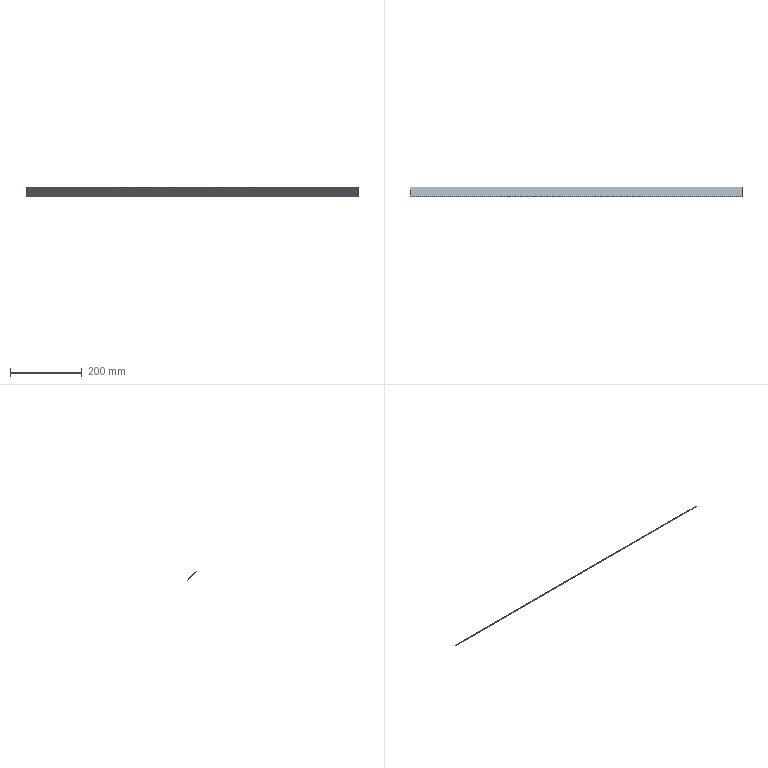Part | SolidWorks | features BaseBody 1 | 1 solid | 6 faces | box 924.6 x 26.8 x 26.8 mm | volume 50484 mm3 | plane 6
STEP:
#1=CARTESIAN_POINT('',(924.6,26.8,2.121));
#2=VERTEX_POINT('',#1);
#3=CARTESIAN_POINT('',(924.6,26.8,0.));
#4=VERTEX_POINT('',#3);
#5=CARTESIAN_POINT('',(924.6,26.8,0.));
#6=DIRECTION('',(0.,0.,-1.));
#7=VECTOR('',#6,1000.);
#8=LINE('',#5,#7);
#9=EDGE_CURVE('',#2,#4,#8,.T.);
#10=ORIENTED_EDGE('',*,*,#9,.T.);
#11=CARTESIAN_POINT('',(0.,26.8,0.));
#12=VERTEX_POINT('',#11);
#13=CARTESIAN_POINT('',(924.6,26.8,0.));
#14=DIRECTION('',(-1.,0.,0.));
#15=VECTOR('',#14,1000.);
#16=LINE('',#13,#15);
#17=EDGE_CURVE('',#4,#12,#16,.T.);
#18=ORIENTED_EDGE('',*,*,#17,.T.);
#19=CARTESIAN_POINT('',(0.,26.8,2.121));
#20=VERTEX_POINT('',#19);
#21=CARTESIAN_POINT('',(0.,26.8,0.));
#22=DIRECTION('',(0.,0.,1.));
#23=VECTOR('',#22,1000.);
#24=LINE('',#21,#23);
#25=EDGE_CURVE('',#12,#20,#24,.T.);
#26=ORIENTED_EDGE('',*,*,#25,.T.);
#27=CARTESIAN_POINT('',(924.6,26.8,2.121));
#28=DIRECTION('',(-1.,0.,0.));
#29=VECTOR('',#28,1000.);
#30=LINE('',#27,#29);
#31=EDGE_CURVE('',#2,#20,#30,.T.);
#32=ORIENTED_EDGE('',*,*,#31,.F.);
#33=EDGE_LOOP('',(#10,#18,#26,#32));
#34=FACE_OUTER_BOUND('',#33,.T.);
#35=CARTESIAN_POINT('',(0.,26.8,0.));
#36=DIRECTION('',(0.,-1.,0.));
#37=DIRECTION('',(0.,0.,-1.));
#38=AXIS2_PLACEMENT_3D('',#35,#36,#37);
#39=PLANE('',#38);
#40=ADVANCED_FACE('',(#34),#39,.F.);
#41=CARTESIAN_POINT('',(0.,0.,26.8));
#42=VERTEX_POINT('',#41);
#43=CARTESIAN_POINT('',(0.,2.121,26.8));
#44=VERTEX_POINT('',#43);
#45=CARTESIAN_POINT('',(0.,0.,26.8));
#46=DIRECTION('',(0.,1.,0.));
#47=VECTOR('',#46,1000.);
#48=LINE('',#45,#47);
#49=EDGE_CURVE('',#42,#44,#48,.T.);
#50=ORIENTED_EDGE('',*,*,#49,.F.);
#51=CARTESIAN_POINT('',(924.6,0.,26.8));
#52=VERTEX_POINT('',#51);
#53=CARTESIAN_POINT('',(924.6,0.,26.8));
#54=DIRECTION('',(-1.,0.,0.));
#55=VECTOR('',#54,1000.);
#56=LINE('',#53,#55);
#57=EDGE_CURVE('',#52,#42,#56,.T.);
#58=ORIENTED_EDGE('',*,*,#57,.F.);
#59=CARTESIAN_POINT('',(924.6,2.121,26.8));
#60=VERTEX_POINT('',#59);
#61=CARTESIAN_POINT('',(924.6,0.,26.8));
#62=DIRECTION('',(0.,1.,0.));
#63=VECTOR('',#62,1000.);
#64=LINE('',#61,#63);
#65=EDGE_CURVE('',#52,#60,#64,.T.);
#66=ORIENTED_EDGE('',*,*,#65,.T.);
#67=CARTESIAN_POINT('',(924.6,2.121,26.8));
#68=DIRECTION('',(1.,0.,0.));
#69=VECTOR('',#68,1000.);
#70=LINE('',#67,#69);
#71=EDGE_CURVE('',#44,#60,#70,.T.);
#72=ORIENTED_EDGE('',*,*,#71,.F.);
#73=EDGE_LOOP('',(#50,#58,#66,#72));
#74=FACE_OUTER_BOUND('',#73,.T.);
#75=CARTESIAN_POINT('',(0.,0.,26.8));
#76=DIRECTION('',(0.,0.,-1.));
#77=DIRECTION('',(0.,-1.,0.));
#78=AXIS2_PLACEMENT_3D('',#75,#76,#77);
#79=PLANE('',#78);
#80=ADVANCED_FACE('',(#74),#79,.F.);
#81=ORIENTED_EDGE('',*,*,#25,.F.);
#82=CARTESIAN_POINT('',(0.,26.8,0.));
#83=DIRECTION('',(0.,-0.7071,0.7071));
#84=VECTOR('',#83,1000.);
#85=LINE('',#82,#84);
#86=EDGE_CURVE('',#12,#42,#85,.T.);
#87=ORIENTED_EDGE('',*,*,#86,.T.);
#88=ORIENTED_EDGE('',*,*,#49,.T.);
#89=CARTESIAN_POINT('',(0.,27.861,1.061));
#90=DIRECTION('',(0.,-0.7071,0.7071));
#91=VECTOR('',#90,1000.);
#92=LINE('',#89,#91);
#93=EDGE_CURVE('',#20,#44,#92,.T.);
#94=ORIENTED_EDGE('',*,*,#93,.F.);
#95=EDGE_LOOP('',(#81,#87,#88,#94));
#96=FACE_OUTER_BOUND('',#95,.T.);
#97=CARTESIAN_POINT('',(0.,0.,0.));
#98=DIRECTION('',(-1.,0.,0.));
#99=DIRECTION('',(0.,0.,1.));
#100=AXIS2_PLACEMENT_3D('',#97,#98,#99);
#101=PLANE('',#100);
#102=ADVANCED_FACE('',(#96),#101,.T.);
#103=CARTESIAN_POINT('',(924.6,26.8,0.));
#104=DIRECTION('',(0.,-0.7071,0.7071));
#105=VECTOR('',#104,1000.);
#106=LINE('',#103,#105);
#107=EDGE_CURVE('',#4,#52,#106,.T.);
#108=ORIENTED_EDGE('',*,*,#107,.F.);
#109=ORIENTED_EDGE('',*,*,#9,.F.);
#110=CARTESIAN_POINT('',(924.6,27.861,1.061));
#111=DIRECTION('',(0.,-0.7071,0.7071));
#112=VECTOR('',#111,1000.);
#113=LINE('',#110,#112);
#114=EDGE_CURVE('',#2,#60,#113,.T.);
#115=ORIENTED_EDGE('',*,*,#114,.T.);
#116=ORIENTED_EDGE('',*,*,#65,.F.);
#117=EDGE_LOOP('',(#108,#109,#115,#116));
#118=FACE_OUTER_BOUND('',#117,.T.);
#119=CARTESIAN_POINT('',(924.6,0.,0.));
#120=DIRECTION('',(-1.,0.,0.));
#121=DIRECTION('',(0.,0.,1.));
#122=AXIS2_PLACEMENT_3D('',#119,#120,#121);
#123=PLANE('',#122);
#124=ADVANCED_FACE('',(#118),#123,.F.);
#125=ORIENTED_EDGE('',*,*,#86,.F.);
#126=ORIENTED_EDGE('',*,*,#17,.F.);
#127=ORIENTED_EDGE('',*,*,#107,.T.);
#128=ORIENTED_EDGE('',*,*,#57,.T.);
#129=EDGE_LOOP('',(#125,#126,#127,#128));
#130=FACE_OUTER_BOUND('',#129,.T.);
#131=CARTESIAN_POINT('',(924.6,26.8,0.));
#132=DIRECTION('',(0.,-0.7071,-0.7071));
#133=DIRECTION('',(0.,-0.7071,0.7071));
#134=AXIS2_PLACEMENT_3D('',#131,#132,#133);
#135=PLANE('',#134);
#136=ADVANCED_FACE('',(#130),#135,.T.);
#137=ORIENTED_EDGE('',*,*,#114,.F.);
#138=ORIENTED_EDGE('',*,*,#31,.T.);
#139=ORIENTED_EDGE('',*,*,#93,.T.);
#140=ORIENTED_EDGE('',*,*,#71,.T.);
#141=EDGE_LOOP('',(#137,#138,#139,#140));
#142=FACE_OUTER_BOUND('',#141,.T.);
#143=CARTESIAN_POINT('',(924.6,27.861,1.061));
#144=DIRECTION('',(0.,-0.7071,-0.7071));
#145=DIRECTION('',(0.,-0.7071,0.7071));
#146=AXIS2_PLACEMENT_3D('',#143,#144,#145);
#147=PLANE('',#146);
#148=ADVANCED_FACE('',(#142),#147,.F.);
#149=CLOSED_SHELL('',(#40,#80,#102,#124,#136,#148));
#150=MANIFOLD_SOLID_BREP('',#149);
#151=CARTESIAN_POINT('',(0.,0.,0.));
#152=DIRECTION('',(0.,0.,1.));
#153=DIRECTION('',(1.,0.,0.));
#154=AXIS2_PLACEMENT_3D('',#151,#152,#153);
#155=(LENGTH_UNIT()NAMED_UNIT(*)SI_UNIT(.MILLI.,.METRE.));
#156=UNCERTAINTY_MEASURE_WITH_UNIT(LENGTH_MEASURE(0.00001),#155,'','');
#157=(NAMED_UNIT(*)PLANE_ANGLE_UNIT()SI_UNIT($,.RADIAN.));
#158=(NAMED_UNIT(*)SI_UNIT($,.STERADIAN.)SOLID_ANGLE_UNIT());
#159=(GEOMETRIC_REPRESENTATION_CONTEXT(3)GLOBAL_UNCERTAINTY_ASSIGNED_CONTEXT((#156))GLOBAL_UNIT_ASSIGNED_CONTEXT((#155,#157,#158))REPRESENTATION_CONTEXT('',''));
#160=ADVANCED_BREP_SHAPE_REPRESENTATION('',(#150,#154),#159);